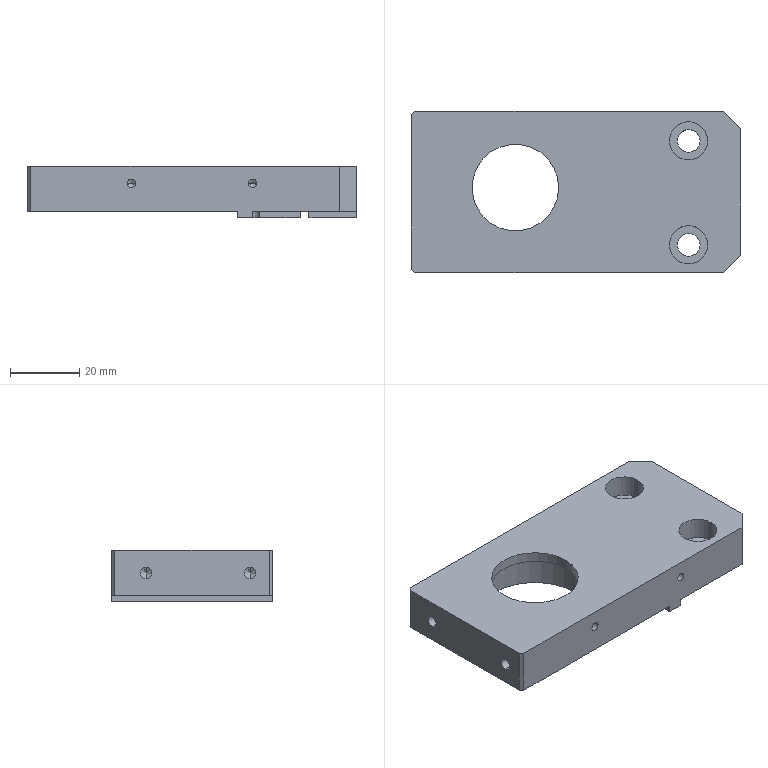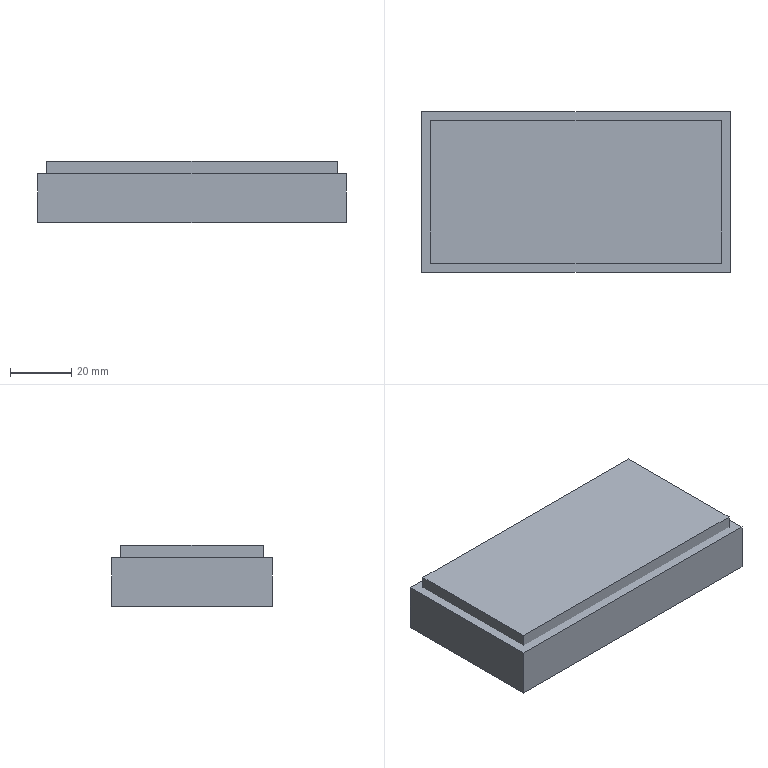CAM job | NX | 3-axis milling, drilling | part box 95 x 46.5 x 15 mm | stock box 101 x 52.5 x 20 mm
Tools:
number,name,description,diameter,corner_radius,flute_length,length,flutes
1,D63,Milling Tool-5 Parameters,63.0,0.0,50.0,75.0,2
10,D10,Milling Tool-5 Parameters,10.0,0.0,50.0,75.0,2
7,D6A45,Milling Tool-5 Parameters,6.0,0.0,3.0,3.0,2
16,6.6ZT,Drilling Tool,6.6,0.0,35.0,50.0,2
4,D4,Milling Tool-5 Parameters,4.0,0.0,50.0,75.0,2
6,D6,Milling Tool-5 Parameters,6.0,0.0,50.0,75.0,2
11,D10JING,Milling Tool-5 Parameters,10.0,0.0,50.0,75.0,2
2,D2,Milling Tool-5 Parameters,2.0,0.0,50.0,75.0,2
Operations:
program,operation,operation_type,tool,method,geometry_group,spindle_rpm,surface_speed,feed_per_tooth,feed_cut,feed_plunge,cut_length_mm,path_length_mm,cut_time_min,machine_time_min
1-98-50-20毛胚,FLOOR_WALL,VolumeBased25DMillingOperation,D63,METHOD,A,6500.0,1286.0,0.0962,1250.0,100.0,176.0,230.0,0.1408,0.1462
1-98-50-20毛胚,DRILLING_COPY_1,Operation,D6A45,METHOD,A,3000.0,56.0,0.0333,200.0,0.0,15.15,179.187,0.0757,0.0922
1-98-50-20毛胚,DRILLING_COPY_1_COPY_COPY_2,Operation,6.6ZT,METHOD,A,2000.0,15.0,0.0375,150.0,0.0,59.949,268.784,0.3997,0.4205
1-98-50-20毛胚,ADAPTIVE_MILLING,CavityMilling,D10,METHOD,A,7000.0,219.0,0.2143,3000.0,1000.0,2715.258,2901.527,1.595,1.613
1-98-50-20毛胚,HOLE_MILLING,CylinderMilling,D6,METHOD,A,7000.0,131.0,0.1071,1500.0,100.0,589.224,751.024,0.3928,0.409
1-98-50-20毛胚,ZLEVEL_PROFILE_COPY_COPY_1_COPY_COPY_COPY_1,ZLevelMilling,D10JING,METHOD,A,7000.0,219.0,0.0714,1000.0,100.0,361.334,579.907,0.3613,0.3832
1-98-50-20毛胚,ZLEVEL_PROFILE_COPY_1_COPY_COPY_COPY_COPY_2_COPY,ZLevelMilling,D6A45,METHOD,A,7000.0,131.0,0.0714,1000.0,1000.0,425.766,825.089,0.4258,0.4657
2-98-50-20毛胚,FLOOR_WALL_1,VolumeBased25DMillingOperation,D63,METHOD,B,6500.0,1286.0,0.0962,1250.0,100.0,850.0,1756.001,0.68,0.7706
2-98-50-20毛胚,FLOOR_WALL_2,VolumeBased25DMillingOperation,D10,METHOD,B,7500.0,235.0,0.1667,2500.0,1000.0,1792.208,2274.467,0.7347,0.7829
2-98-50-20毛胚,HOLE_MILLING_COPY,CylinderMilling,D10,METHOD,B,7000.0,219.0,0.1071,1500.0,100.0,819.912,893.412,0.5466,0.554
2-98-50-20毛胚,ZLEVEL_PROFILE_COPY_1,ZLevelMilling,D4,METHOD,B,7000.0,87.0,0.1071,1500.0,1000.0,171.905,509.951,0.1204,0.1542
2-98-50-20毛胚,FLOOR_WALL_1_COPY_1,VolumeBased25DMillingOperation,D4,METHOD,B,7000.0,87.0,0.0714,1000.0,100.0,2237.302,2792.908,2.237,2.3
2-98-50-20毛胚,ZLEVEL_PROFILE_COPY_1_COPY,ZLevelMilling,D2,METHOD,B,7000.0,43.0,0.0714,1000.0,1000.0,313.432,672.579,0.3134,0.3493
2-98-50-20毛胚,ZLEVEL_PROFILE_COPY_1_COPY_COPY_COPY_COPY_2_COPY_COPY,ZLevelMilling,D6A45,METHOD,B,7000.0,131.0,0.0714,1000.0,1000.0,282.639,546.199,0.2826,0.309
2-98-50-20毛胚,ZLEVEL_PROFILE_COPY_1_COPY_COPY_COPY_COPY_2_COPY_COPY_COPY,ZLevelMilling,D6A45,METHOD,B,7000.0,131.0,0.0714,1000.0,1000.0,343.424,780.719,0.3434,0.3872
2-98-50-20毛胚,刀补11,CylinderMilling,D10JING,METHOD,B,7000.0,219.0,0.0714,1000.0,100.0,193.075,279.35,0.1931,0.2017